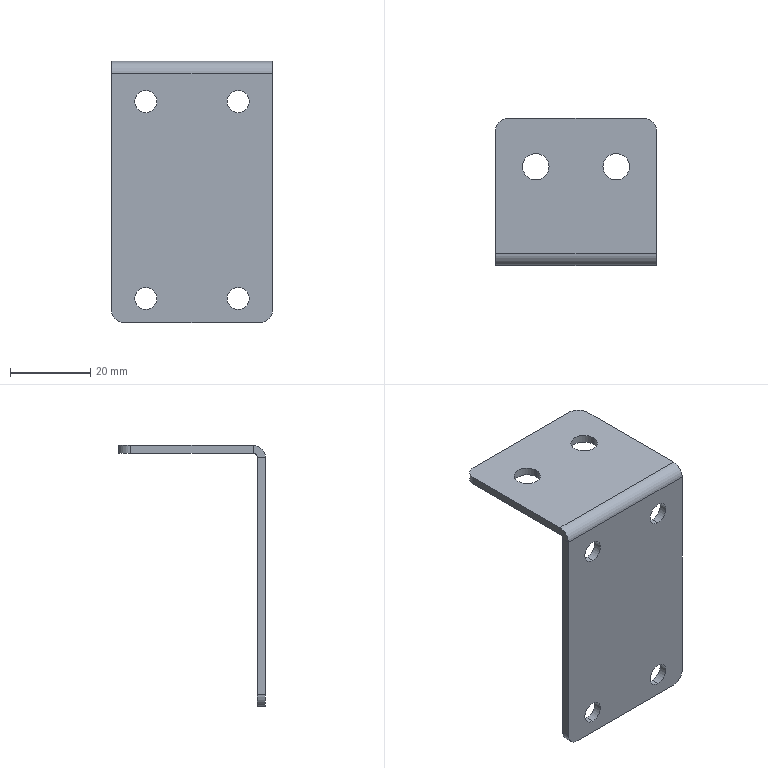Part | SolidWorks | features HoleWzd 2, Fillet 1, FlatPattern 1, SMBaseFlange 1, SheetMetal 1 | 1 solid | 30 faces | box 40 x 36.5 x 65 mm | volume 7549 mm3 | cylinder 18 | plane 12 | commonest cylinder face diameters 5.5 x8 6 x5 6.6 x4 2 x1
STEP:
#1=CARTESIAN_POINT('',(31.5,2.,-56.25));
#2=VERTEX_POINT('',#1);
#3=CARTESIAN_POINT('',(31.5,2.,-61.75));
#4=VERTEX_POINT('',#3);
#5=CARTESIAN_POINT('',(31.5,2.,-59.));
#6=DIRECTION('',(0.,-1.,0.));
#7=DIRECTION('',(0.,0.,-1.));
#8=AXIS2_PLACEMENT_3D('',#5,#6,#7);
#9=CIRCLE('',#8,2.75);
#10=EDGE_CURVE('',#2,#4,#9,.T.);
#11=ORIENTED_EDGE('',*,*,#10,.F.);
#12=CARTESIAN_POINT('',(31.5,0.,-56.25));
#13=VERTEX_POINT('',#12);
#14=CARTESIAN_POINT('',(31.5,0.,-56.25));
#15=DIRECTION('',(0.,-1.,0.));
#16=VECTOR('',#15,1000.);
#17=LINE('',#14,#16);
#18=EDGE_CURVE('',#2,#13,#17,.T.);
#19=ORIENTED_EDGE('',*,*,#18,.T.);
#20=CARTESIAN_POINT('',(31.5,0.,-61.75));
#21=VERTEX_POINT('',#20);
#22=CARTESIAN_POINT('',(31.5,0.,-59.));
#23=DIRECTION('',(0.,-1.,0.));
#24=DIRECTION('',(0.,0.,-1.));
#25=AXIS2_PLACEMENT_3D('',#22,#23,#24);
#26=CIRCLE('',#25,2.75);
#27=EDGE_CURVE('',#13,#21,#26,.T.);
#28=ORIENTED_EDGE('',*,*,#27,.T.);
#29=CARTESIAN_POINT('',(31.5,0.,-61.75));
#30=DIRECTION('',(0.,-1.,0.));
#31=VECTOR('',#30,1000.);
#32=LINE('',#29,#31);
#33=EDGE_CURVE('',#4,#21,#32,.T.);
#34=ORIENTED_EDGE('',*,*,#33,.F.);
#35=EDGE_LOOP('',(#11,#19,#28,#34));
#36=FACE_OUTER_BOUND('',#35,.T.);
#37=CARTESIAN_POINT('',(31.5,0.,-59.));
#38=DIRECTION('',(0.,-1.,0.));
#39=DIRECTION('',(0.,0.,-1.));
#40=AXIS2_PLACEMENT_3D('',#37,#38,#39);
#41=CYLINDRICAL_SURFACE('',#40,2.75);
#42=ADVANCED_FACE('',(#36),#41,.F.);
#43=CARTESIAN_POINT('',(31.5,2.,-7.25));
#44=VERTEX_POINT('',#43);
#45=CARTESIAN_POINT('',(31.5,2.,-12.75));
#46=VERTEX_POINT('',#45);
#47=CARTESIAN_POINT('',(31.5,2.,-10.));
#48=DIRECTION('',(0.,-1.,0.));
#49=DIRECTION('',(0.,0.,-1.));
#50=AXIS2_PLACEMENT_3D('',#47,#48,#49);
#51=CIRCLE('',#50,2.75);
#52=EDGE_CURVE('',#44,#46,#51,.T.);
#53=ORIENTED_EDGE('',*,*,#52,.F.);
#54=CARTESIAN_POINT('',(31.5,0.,-7.25));
#55=VERTEX_POINT('',#54);
#56=CARTESIAN_POINT('',(31.5,0.,-7.25));
#57=DIRECTION('',(0.,-1.,0.));
#58=VECTOR('',#57,1000.);
#59=LINE('',#56,#58);
#60=EDGE_CURVE('',#44,#55,#59,.T.);
#61=ORIENTED_EDGE('',*,*,#60,.T.);
#62=CARTESIAN_POINT('',(31.5,0.,-12.75));
#63=VERTEX_POINT('',#62);
#64=CARTESIAN_POINT('',(31.5,0.,-10.));
#65=DIRECTION('',(0.,-1.,0.));
#66=DIRECTION('',(0.,0.,-1.));
#67=AXIS2_PLACEMENT_3D('',#64,#65,#66);
#68=CIRCLE('',#67,2.75);
#69=EDGE_CURVE('',#55,#63,#68,.T.);
#70=ORIENTED_EDGE('',*,*,#69,.T.);
#71=CARTESIAN_POINT('',(31.5,0.,-12.75));
#72=DIRECTION('',(0.,-1.,0.));
#73=VECTOR('',#72,1000.);
#74=LINE('',#71,#73);
#75=EDGE_CURVE('',#46,#63,#74,.T.);
#76=ORIENTED_EDGE('',*,*,#75,.F.);
#77=EDGE_LOOP('',(#53,#61,#70,#76));
#78=FACE_OUTER_BOUND('',#77,.T.);
#79=CARTESIAN_POINT('',(31.5,0.,-10.));
#80=DIRECTION('',(0.,-1.,0.));
#81=DIRECTION('',(0.,0.,-1.));
#82=AXIS2_PLACEMENT_3D('',#79,#80,#81);
#83=CYLINDRICAL_SURFACE('',#82,2.75);
#84=ADVANCED_FACE('',(#78),#83,.F.);
#85=CARTESIAN_POINT('',(8.5,2.,-7.25));
#86=VERTEX_POINT('',#85);
#87=CARTESIAN_POINT('',(8.5,2.,-12.75));
#88=VERTEX_POINT('',#87);
#89=CARTESIAN_POINT('',(8.5,2.,-10.));
#90=DIRECTION('',(0.,-1.,0.));
#91=DIRECTION('',(0.,0.,-1.));
#92=AXIS2_PLACEMENT_3D('',#89,#90,#91);
#93=CIRCLE('',#92,2.75);
#94=EDGE_CURVE('',#86,#88,#93,.T.);
#95=ORIENTED_EDGE('',*,*,#94,.F.);
#96=CARTESIAN_POINT('',(8.5,0.,-7.25));
#97=VERTEX_POINT('',#96);
#98=CARTESIAN_POINT('',(8.5,0.,-7.25));
#99=DIRECTION('',(0.,-1.,0.));
#100=VECTOR('',#99,1000.);
#101=LINE('',#98,#100);
#102=EDGE_CURVE('',#86,#97,#101,.T.);
#103=ORIENTED_EDGE('',*,*,#102,.T.);
#104=CARTESIAN_POINT('',(8.5,0.,-12.75));
#105=VERTEX_POINT('',#104);
#106=CARTESIAN_POINT('',(8.5,0.,-10.));
#107=DIRECTION('',(0.,-1.,0.));
#108=DIRECTION('',(0.,0.,-1.));
#109=AXIS2_PLACEMENT_3D('',#106,#107,#108);
#110=CIRCLE('',#109,2.75);
#111=EDGE_CURVE('',#97,#105,#110,.T.);
#112=ORIENTED_EDGE('',*,*,#111,.T.);
#113=CARTESIAN_POINT('',(8.5,0.,-12.75));
#114=DIRECTION('',(0.,-1.,0.));
#115=VECTOR('',#114,1000.);
#116=LINE('',#113,#115);
#117=EDGE_CURVE('',#88,#105,#116,.T.);
#118=ORIENTED_EDGE('',*,*,#117,.F.);
#119=EDGE_LOOP('',(#95,#103,#112,#118));
#120=FACE_OUTER_BOUND('',#119,.T.);
#121=CARTESIAN_POINT('',(8.5,0.,-10.));
#122=DIRECTION('',(0.,-1.,0.));
#123=DIRECTION('',(0.,0.,-1.));
#124=AXIS2_PLACEMENT_3D('',#121,#122,#123);
#125=CYLINDRICAL_SURFACE('',#124,2.75);
#126=ADVANCED_FACE('',(#120),#125,.F.);
#127=CARTESIAN_POINT('',(8.5,2.,-56.25));
#128=VERTEX_POINT('',#127);
#129=CARTESIAN_POINT('',(8.5,2.,-61.75));
#130=VERTEX_POINT('',#129);
#131=CARTESIAN_POINT('',(8.5,2.,-59.));
#132=DIRECTION('',(0.,-1.,0.));
#133=DIRECTION('',(0.,0.,-1.));
#134=AXIS2_PLACEMENT_3D('',#131,#132,#133);
#135=CIRCLE('',#134,2.75);
#136=EDGE_CURVE('',#128,#130,#135,.T.);
#137=ORIENTED_EDGE('',*,*,#136,.F.);
#138=CARTESIAN_POINT('',(8.5,0.,-56.25));
#139=VERTEX_POINT('',#138);
#140=CARTESIAN_POINT('',(8.5,0.,-56.25));
#141=DIRECTION('',(0.,-1.,0.));
#142=VECTOR('',#141,1000.);
#143=LINE('',#140,#142);
#144=EDGE_CURVE('',#128,#139,#143,.T.);
#145=ORIENTED_EDGE('',*,*,#144,.T.);
#146=CARTESIAN_POINT('',(8.5,0.,-61.75));
#147=VERTEX_POINT('',#146);
#148=CARTESIAN_POINT('',(8.5,0.,-59.));
#149=DIRECTION('',(0.,-1.,0.));
#150=DIRECTION('',(0.,0.,-1.));
#151=AXIS2_PLACEMENT_3D('',#148,#149,#150);
#152=CIRCLE('',#151,2.75);
#153=EDGE_CURVE('',#139,#147,#152,.T.);
#154=ORIENTED_EDGE('',*,*,#153,.T.);
#155=CARTESIAN_POINT('',(8.5,0.,-61.75));
#156=DIRECTION('',(0.,-1.,0.));
#157=VECTOR('',#156,1000.);
#158=LINE('',#155,#157);
#159=EDGE_CURVE('',#130,#147,#158,.T.);
#160=ORIENTED_EDGE('',*,*,#159,.F.);
#161=EDGE_LOOP('',(#137,#145,#154,#160));
#162=FACE_OUTER_BOUND('',#161,.T.);
#163=CARTESIAN_POINT('',(8.5,0.,-59.));
#164=DIRECTION('',(0.,-1.,0.));
#165=DIRECTION('',(0.,0.,-1.));
#166=AXIS2_PLACEMENT_3D('',#163,#164,#165);
#167=CYLINDRICAL_SURFACE('',#166,2.75);
#168=ADVANCED_FACE('',(#162),#167,.F.);
#169=CARTESIAN_POINT('',(33.3,24.5,0.));
#170=VERTEX_POINT('',#169);
#171=CARTESIAN_POINT('',(26.7,24.5,0.));
#172=VERTEX_POINT('',#171);
#173=CARTESIAN_POINT('',(30.,24.5,0.));
#174=DIRECTION('',(0.,0.,-1.));
#175=DIRECTION('',(-1.,0.,0.));
#176=AXIS2_PLACEMENT_3D('',#173,#174,#175);
#177=CIRCLE('',#176,3.3);
#178=EDGE_CURVE('',#170,#172,#177,.T.);
#179=ORIENTED_EDGE('',*,*,#178,.F.);
#180=CARTESIAN_POINT('',(33.3,24.5,-2.));
#181=VERTEX_POINT('',#180);
#182=CARTESIAN_POINT('',(33.3,24.5,-2.));
#183=DIRECTION('',(0.,0.,-1.));
#184=VECTOR('',#183,1000.);
#185=LINE('',#182,#184);
#186=EDGE_CURVE('',#170,#181,#185,.T.);
#187=ORIENTED_EDGE('',*,*,#186,.T.);
#188=CARTESIAN_POINT('',(26.7,24.5,-2.));
#189=VERTEX_POINT('',#188);
#190=CARTESIAN_POINT('',(30.,24.5,-2.));
#191=DIRECTION('',(0.,0.,-1.));
#192=DIRECTION('',(-1.,0.,0.));
#193=AXIS2_PLACEMENT_3D('',#190,#191,#192);
#194=CIRCLE('',#193,3.3);
#195=EDGE_CURVE('',#181,#189,#194,.T.);
#196=ORIENTED_EDGE('',*,*,#195,.T.);
#197=CARTESIAN_POINT('',(26.7,24.5,-2.));
#198=DIRECTION('',(0.,0.,-1.));
#199=VECTOR('',#198,1000.);
#200=LINE('',#197,#199);
#201=EDGE_CURVE('',#172,#189,#200,.T.);
#202=ORIENTED_EDGE('',*,*,#201,.F.);
#203=EDGE_LOOP('',(#179,#187,#196,#202));
#204=FACE_OUTER_BOUND('',#203,.T.);
#205=CARTESIAN_POINT('',(30.,24.5,-2.));
#206=DIRECTION('',(0.,0.,-1.));
#207=DIRECTION('',(-1.,0.,0.));
#208=AXIS2_PLACEMENT_3D('',#205,#206,#207);
#209=CYLINDRICAL_SURFACE('',#208,3.3);
#210=ADVANCED_FACE('',(#204),#209,.F.);
#211=CARTESIAN_POINT('',(13.3,24.5,0.));
#212=VERTEX_POINT('',#211);
#213=CARTESIAN_POINT('',(6.7,24.5,0.));
#214=VERTEX_POINT('',#213);
#215=CARTESIAN_POINT('',(10.,24.5,0.));
#216=DIRECTION('',(0.,0.,-1.));
#217=DIRECTION('',(-1.,0.,0.));
#218=AXIS2_PLACEMENT_3D('',#215,#216,#217);
#219=CIRCLE('',#218,3.3);
#220=EDGE_CURVE('',#212,#214,#219,.T.);
#221=ORIENTED_EDGE('',*,*,#220,.F.);
#222=CARTESIAN_POINT('',(13.3,24.5,-2.));
#223=VERTEX_POINT('',#222);
#224=CARTESIAN_POINT('',(13.3,24.5,-2.));
#225=DIRECTION('',(0.,0.,-1.));
#226=VECTOR('',#225,1000.);
#227=LINE('',#224,#226);
#228=EDGE_CURVE('',#212,#223,#227,.T.);
#229=ORIENTED_EDGE('',*,*,#228,.T.);
#230=CARTESIAN_POINT('',(6.7,24.5,-2.));
#231=VERTEX_POINT('',#230);
#232=CARTESIAN_POINT('',(10.,24.5,-2.));
#233=DIRECTION('',(0.,0.,-1.));
#234=DIRECTION('',(-1.,0.,0.));
#235=AXIS2_PLACEMENT_3D('',#232,#233,#234);
#236=CIRCLE('',#235,3.3);
#237=EDGE_CURVE('',#223,#231,#236,.T.);
#238=ORIENTED_EDGE('',*,*,#237,.T.);
#239=CARTESIAN_POINT('',(6.7,24.5,-2.));
#240=DIRECTION('',(0.,0.,-1.));
#241=VECTOR('',#240,1000.);
#242=LINE('',#239,#241);
#243=EDGE_CURVE('',#214,#231,#242,.T.);
#244=ORIENTED_EDGE('',*,*,#243,.F.);
#245=EDGE_LOOP('',(#221,#229,#238,#244));
#246=FACE_OUTER_BOUND('',#245,.T.);
#247=CARTESIAN_POINT('',(10.,24.5,-2.));
#248=DIRECTION('',(0.,0.,-1.));
#249=DIRECTION('',(-1.,0.,0.));
#250=AXIS2_PLACEMENT_3D('',#247,#248,#249);
#251=CYLINDRICAL_SURFACE('',#250,3.3);
#252=ADVANCED_FACE('',(#246),#251,.F.);
#253=CARTESIAN_POINT('',(40.,3.,0.));
#254=VERTEX_POINT('',#253);
#255=CARTESIAN_POINT('',(40.,3.,-2.));
#256=VERTEX_POINT('',#255);
#257=CARTESIAN_POINT('',(40.,3.,0.));
#258=DIRECTION('',(0.,0.,-1.));
#259=VECTOR('',#258,1000.);
#260=LINE('',#257,#259);
#261=EDGE_CURVE('',#254,#256,#260,.T.);
#262=ORIENTED_EDGE('',*,*,#261,.F.);
#263=CARTESIAN_POINT('',(40.,0.,-3.));
#264=VERTEX_POINT('',#263);
#265=CARTESIAN_POINT('',(40.,3.,-3.));
#266=DIRECTION('',(-1.,0.,0.));
#267=DIRECTION('',(0.,0.,-1.));
#268=AXIS2_PLACEMENT_3D('',#265,#266,#267);
#269=CIRCLE('',#268,3.);
#270=EDGE_CURVE('',#264,#254,#269,.T.);
#271=ORIENTED_EDGE('',*,*,#270,.F.);
#272=CARTESIAN_POINT('',(40.,2.,-3.));
#273=VERTEX_POINT('',#272);
#274=CARTESIAN_POINT('',(40.,2.,-3.));
#275=DIRECTION('',(0.,-1.,0.));
#276=VECTOR('',#275,1000.);
#277=LINE('',#274,#276);
#278=EDGE_CURVE('',#273,#264,#277,.T.);
#279=ORIENTED_EDGE('',*,*,#278,.F.);
#280=CARTESIAN_POINT('',(40.,3.,-3.));
#281=DIRECTION('',(-1.,0.,0.));
#282=DIRECTION('',(0.,0.,-1.));
#283=AXIS2_PLACEMENT_3D('',#280,#281,#282);
#284=CIRCLE('',#283,1.);
#285=EDGE_CURVE('',#273,#256,#284,.T.);
#286=ORIENTED_EDGE('',*,*,#285,.T.);
#287=EDGE_LOOP('',(#262,#271,#279,#286));
#288=FACE_OUTER_BOUND('',#287,.T.);
#289=CARTESIAN_POINT('',(40.,3.,0.));
#290=DIRECTION('',(1.,0.,0.));
#291=DIRECTION('',(0.,0.,-1.));
#292=AXIS2_PLACEMENT_3D('',#289,#290,#291);
#293=PLANE('',#292);
#294=ADVANCED_FACE('',(#288),#293,.T.);
#295=CARTESIAN_POINT('',(40.,33.5,-2.));
#296=VERTEX_POINT('',#295);
#297=CARTESIAN_POINT('',(40.,0.,-2.));
#298=DIRECTION('',(0.,1.,0.));
#299=VECTOR('',#298,1000.);
#300=LINE('',#297,#299);
#301=EDGE_CURVE('',#256,#296,#300,.T.);
#302=ORIENTED_EDGE('',*,*,#301,.T.);
#303=CARTESIAN_POINT('',(40.,33.5,0.));
#304=VERTEX_POINT('',#303);
#305=CARTESIAN_POINT('',(40.,33.5,-3.));
#306=DIRECTION('',(0.,0.,1.));
#307=VECTOR('',#306,1000.);
#308=LINE('',#305,#307);
#309=EDGE_CURVE('',#296,#304,#308,.T.);
#310=ORIENTED_EDGE('',*,*,#309,.T.);
#311=CARTESIAN_POINT('',(40.,0.,0.));
#312=DIRECTION('',(0.,1.,0.));
#313=VECTOR('',#312,1000.);
#314=LINE('',#311,#313);
#315=EDGE_CURVE('',#254,#304,#314,.T.);
#316=ORIENTED_EDGE('',*,*,#315,.F.);
#317=ORIENTED_EDGE('',*,*,#261,.T.);
#318=EDGE_LOOP('',(#302,#310,#316,#317));
#319=FACE_OUTER_BOUND('',#318,.T.);
#320=CARTESIAN_POINT('',(40.,2.,-3.));
#321=DIRECTION('',(1.,0.,0.));
#322=DIRECTION('',(0.,0.,-1.));
#323=AXIS2_PLACEMENT_3D('',#320,#321,#322);
#324=PLANE('',#323);
#325=ADVANCED_FACE('',(#319),#324,.T.);
#326=CARTESIAN_POINT('',(0.,0.,-3.));
#327=VERTEX_POINT('',#326);
#328=CARTESIAN_POINT('',(0.,2.,-3.));
#329=VERTEX_POINT('',#328);
#330=CARTESIAN_POINT('',(0.,0.,-3.));
#331=DIRECTION('',(0.,1.,0.));
#332=VECTOR('',#331,1000.);
#333=LINE('',#330,#332);
#334=EDGE_CURVE('',#327,#329,#333,.T.);
#335=ORIENTED_EDGE('',*,*,#334,.F.);
#336=CARTESIAN_POINT('',(0.,3.,0.));
#337=VERTEX_POINT('',#336);
#338=CARTESIAN_POINT('',(0.,3.,-3.));
#339=DIRECTION('',(-1.,0.,0.));
#340=DIRECTION('',(0.,0.,-1.));
#341=AXIS2_PLACEMENT_3D('',#338,#339,#340);
#342=CIRCLE('',#341,3.);
#343=EDGE_CURVE('',#327,#337,#342,.T.);
#344=ORIENTED_EDGE('',*,*,#343,.T.);
#345=CARTESIAN_POINT('',(0.,3.,-2.));
#346=VERTEX_POINT('',#345);
#347=CARTESIAN_POINT('',(0.,3.,-2.));
#348=DIRECTION('',(0.,0.,1.));
#349=VECTOR('',#348,1000.);
#350=LINE('',#347,#349);
#351=EDGE_CURVE('',#346,#337,#350,.T.);
#352=ORIENTED_EDGE('',*,*,#351,.F.);
#353=CARTESIAN_POINT('',(0.,3.,-3.));
#354=DIRECTION('',(-1.,0.,0.));
#355=DIRECTION('',(0.,0.,-1.));
#356=AXIS2_PLACEMENT_3D('',#353,#354,#355);
#357=CIRCLE('',#356,1.);
#358=EDGE_CURVE('',#329,#346,#357,.T.);
#359=ORIENTED_EDGE('',*,*,#358,.F.);
#360=EDGE_LOOP('',(#335,#344,#352,#359));
#361=FACE_OUTER_BOUND('',#360,.T.);
#362=CARTESIAN_POINT('',(0.,0.,-3.));
#363=DIRECTION('',(-1.,0.,0.));
#364=DIRECTION('',(0.,0.,1.));
#365=AXIS2_PLACEMENT_3D('',#362,#363,#364);
#366=PLANE('',#365);
#367=ADVANCED_FACE('',(#361),#366,.T.);
#368=CARTESIAN_POINT('',(0.,2.,-62.));
#369=VERTEX_POINT('',#368);
#370=CARTESIAN_POINT('',(0.,2.,0.));
#371=DIRECTION('',(0.,0.,1.));
#372=VECTOR('',#371,1000.);
#373=LINE('',#370,#372);
#374=EDGE_CURVE('',#369,#329,#373,.T.);
#375=ORIENTED_EDGE('',*,*,#374,.F.);
#376=CARTESIAN_POINT('',(0.,0.,-62.));
#377=VERTEX_POINT('',#376);
#378=CARTESIAN_POINT('',(0.,3.,-62.));
#379=DIRECTION('',(0.,-1.,0.));
#380=VECTOR('',#379,1000.);
#381=LINE('',#378,#380);
#382=EDGE_CURVE('',#369,#377,#381,.T.);
#383=ORIENTED_EDGE('',*,*,#382,.T.);
#384=CARTESIAN_POINT('',(0.,0.,0.));
#385=DIRECTION('',(0.,0.,1.));
#386=VECTOR('',#385,1000.);
#387=LINE('',#384,#386);
#388=EDGE_CURVE('',#377,#327,#387,.T.);
#389=ORIENTED_EDGE('',*,*,#388,.T.);
#390=ORIENTED_EDGE('',*,*,#334,.T.);
#391=EDGE_LOOP('',(#375,#383,#389,#390));
#392=FACE_OUTER_BOUND('',#391,.T.);
#393=CARTESIAN_POINT('',(0.,3.,-2.));
#394=DIRECTION('',(-1.,0.,0.));
#395=DIRECTION('',(0.,0.,1.));
#396=AXIS2_PLACEMENT_3D('',#393,#394,#395);
#397=PLANE('',#396);
#398=ADVANCED_FACE('',(#392),#397,.T.);
#399=CARTESIAN_POINT('',(30.,24.5,-2.));
#400=DIRECTION('',(0.,0.,-1.));
#401=DIRECTION('',(-1.,0.,0.));
#402=AXIS2_PLACEMENT_3D('',#399,#400,#401);
#403=CIRCLE('',#402,3.3);
#404=EDGE_CURVE('',#189,#181,#403,.T.);
#405=ORIENTED_EDGE('',*,*,#404,.F.);
#406=ORIENTED_EDGE('',*,*,#195,.F.);
#407=EDGE_LOOP('',(#405,#406));
#408=FACE_BOUND('',#407,.T.);
#409=CARTESIAN_POINT('',(10.,24.5,-2.));
#410=DIRECTION('',(0.,0.,-1.));
#411=DIRECTION('',(-1.,0.,0.));
#412=AXIS2_PLACEMENT_3D('',#409,#410,#411);
#413=CIRCLE('',#412,3.3);
#414=EDGE_CURVE('',#231,#223,#413,.T.);
#415=ORIENTED_EDGE('',*,*,#414,.F.);
#416=ORIENTED_EDGE('',*,*,#237,.F.);
#417=EDGE_LOOP('',(#415,#416));
#418=FACE_BOUND('',#417,.T.);
#419=CARTESIAN_POINT('',(37.,36.5,-2.));
#420=VERTEX_POINT('',#419);
#421=CARTESIAN_POINT('',(3.,36.5,-2.));
#422=VERTEX_POINT('',#421);
#423=CARTESIAN_POINT('',(40.,36.5,-2.));
#424=DIRECTION('',(-1.,0.,0.));
#425=VECTOR('',#424,1000.);
#426=LINE('',#423,#425);
#427=EDGE_CURVE('',#420,#422,#426,.T.);
#428=ORIENTED_EDGE('',*,*,#427,.F.);
#429=CARTESIAN_POINT('',(37.,33.5,-2.));
#430=DIRECTION('',(0.,0.,-1.));
#431=DIRECTION('',(1.,0.,0.));
#432=AXIS2_PLACEMENT_3D('',#429,#430,#431);
#433=CIRCLE('',#432,3.);
#434=EDGE_CURVE('',#420,#296,#433,.T.);
#435=ORIENTED_EDGE('',*,*,#434,.T.);
#436=ORIENTED_EDGE('',*,*,#301,.F.);
#437=CARTESIAN_POINT('',(40.,3.,-2.));
#438=DIRECTION('',(-1.,0.,0.));
#439=VECTOR('',#438,1000.);
#440=LINE('',#437,#439);
#441=EDGE_CURVE('',#256,#346,#440,.T.);
#442=ORIENTED_EDGE('',*,*,#441,.T.);
#443=CARTESIAN_POINT('',(0.,33.5,-2.));
#444=VERTEX_POINT('',#443);
#445=CARTESIAN_POINT('',(0.,0.,-2.));
#446=DIRECTION('',(0.,1.,0.));
#447=VECTOR('',#446,1000.);
#448=LINE('',#445,#447);
#449=EDGE_CURVE('',#346,#444,#448,.T.);
#450=ORIENTED_EDGE('',*,*,#449,.T.);
#451=CARTESIAN_POINT('',(3.,33.5,-2.));
#452=DIRECTION('',(0.,0.,-1.));
#453=DIRECTION('',(1.,0.,0.));
#454=AXIS2_PLACEMENT_3D('',#451,#452,#453);
#455=CIRCLE('',#454,3.);
#456=EDGE_CURVE('',#444,#422,#455,.T.);
#457=ORIENTED_EDGE('',*,*,#456,.T.);
#458=EDGE_LOOP('',(#428,#435,#436,#442,#450,#457));
#459=FACE_OUTER_BOUND('',#458,.T.);
#460=CARTESIAN_POINT('',(40.,0.,-2.));
#461=DIRECTION('',(0.,0.,1.));
#462=DIRECTION('',(1.,0.,0.));
#463=AXIS2_PLACEMENT_3D('',#460,#461,#462);
#464=PLANE('',#463);
#465=ADVANCED_FACE('',(#408,#418,#459),#464,.F.);
#466=CARTESIAN_POINT('',(37.,36.5,0.));
#467=VERTEX_POINT('',#466);
#468=CARTESIAN_POINT('',(3.,36.5,0.));
#469=VERTEX_POINT('',#468);
#470=CARTESIAN_POINT('',(40.,36.5,0.));
#471=DIRECTION('',(-1.,0.,0.));
#472=VECTOR('',#471,1000.);
#473=LINE('',#470,#472);
#474=EDGE_CURVE('',#467,#469,#473,.T.);
#475=ORIENTED_EDGE('',*,*,#474,.F.);
#476=CARTESIAN_POINT('',(37.,36.5,0.));
#477=DIRECTION('',(0.,0.,-1.));
#478=VECTOR('',#477,1000.);
#479=LINE('',#476,#478);
#480=EDGE_CURVE('',#467,#420,#479,.T.);
#481=ORIENTED_EDGE('',*,*,#480,.T.);
#482=ORIENTED_EDGE('',*,*,#427,.T.);
#483=CARTESIAN_POINT('',(3.,36.5,0.));
#484=DIRECTION('',(0.,0.,1.));
#485=VECTOR('',#484,1000.);
#486=LINE('',#483,#485);
#487=EDGE_CURVE('',#422,#469,#486,.T.);
#488=ORIENTED_EDGE('',*,*,#487,.T.);
#489=EDGE_LOOP('',(#475,#481,#482,#488));
#490=FACE_OUTER_BOUND('',#489,.T.);
#491=CARTESIAN_POINT('',(40.,36.5,0.));
#492=DIRECTION('',(0.,1.,0.));
#493=DIRECTION('',(0.,0.,1.));
#494=AXIS2_PLACEMENT_3D('',#491,#492,#493);
#495=PLANE('',#494);
#496=ADVANCED_FACE('',(#490),#495,.T.);
#497=CARTESIAN_POINT('',(30.,24.5,0.));
#498=DIRECTION('',(0.,0.,-1.));
#499=DIRECTION('',(-1.,0.,0.));
#500=AXIS2_PLACEMENT_3D('',#497,#498,#499);
#501=CIRCLE('',#500,3.3);
#502=EDGE_CURVE('',#172,#170,#501,.T.);
#503=ORIENTED_EDGE('',*,*,#502,.T.);
#504=ORIENTED_EDGE('',*,*,#178,.T.);
#505=EDGE_LOOP('',(#503,#504));
#506=FACE_BOUND('',#505,.T.);
#507=CARTESIAN_POINT('',(10.,24.5,0.));
#508=DIRECTION('',(0.,0.,-1.));
#509=DIRECTION('',(-1.,0.,0.));
#510=AXIS2_PLACEMENT_3D('',#507,#508,#509);
#511=CIRCLE('',#510,3.3);
#512=EDGE_CURVE('',#214,#212,#511,.T.);
#513=ORIENTED_EDGE('',*,*,#512,.T.);
#514=ORIENTED_EDGE('',*,*,#220,.T.);
#515=EDGE_LOOP('',(#513,#514));
#516=FACE_BOUND('',#515,.T.);
#517=ORIENTED_EDGE('',*,*,#315,.T.);
#518=CARTESIAN_POINT('',(37.,33.5,0.));
#519=DIRECTION('',(0.,0.,1.));
#520=DIRECTION('',(1.,0.,0.));
#521=AXIS2_PLACEMENT_3D('',#518,#519,#520);
#522=CIRCLE('',#521,3.);
#523=EDGE_CURVE('',#304,#467,#522,.T.);
#524=ORIENTED_EDGE('',*,*,#523,.T.);
#525=ORIENTED_EDGE('',*,*,#474,.T.);
#526=CARTESIAN_POINT('',(0.,33.5,0.));
#527=VERTEX_POINT('',#526);
#528=CARTESIAN_POINT('',(3.,33.5,0.));
#529=DIRECTION('',(0.,0.,1.));
#530=DIRECTION('',(1.,0.,0.));
#531=AXIS2_PLACEMENT_3D('',#528,#529,#530);
#532=CIRCLE('',#531,3.);
#533=EDGE_CURVE('',#469,#527,#532,.T.);
#534=ORIENTED_EDGE('',*,*,#533,.T.);
#535=CARTESIAN_POINT('',(0.,0.,0.));
#536=DIRECTION('',(0.,1.,0.));
#537=VECTOR('',#536,1000.);
#538=LINE('',#535,#537);
#539=EDGE_CURVE('',#337,#527,#538,.T.);
#540=ORIENTED_EDGE('',*,*,#539,.F.);
#541=CARTESIAN_POINT('',(40.,3.,0.));
#542=DIRECTION('',(-1.,0.,0.));
#543=VECTOR('',#542,1000.);
#544=LINE('',#541,#543);
#545=EDGE_CURVE('',#254,#337,#544,.T.);
#546=ORIENTED_EDGE('',*,*,#545,.F.);
#547=EDGE_LOOP('',(#517,#524,#525,#534,#540,#546));
#548=FACE_OUTER_BOUND('',#547,.T.);
#549=CARTESIAN_POINT('',(40.,0.,0.));
#550=DIRECTION('',(0.,0.,1.));
#551=DIRECTION('',(1.,0.,0.));
#552=AXIS2_PLACEMENT_3D('',#549,#550,#551);
#553=PLANE('',#552);
#554=ADVANCED_FACE('',(#506,#516,#548),#553,.T.);
#555=ORIENTED_EDGE('',*,*,#343,.F.);
#556=CARTESIAN_POINT('',(40.,0.,-3.));
#557=DIRECTION('',(-1.,0.,0.));
#558=VECTOR('',#557,1000.);
#559=LINE('',#556,#558);
#560=EDGE_CURVE('',#264,#327,#559,.T.);
#561=ORIENTED_EDGE('',*,*,#560,.F.);
#562=ORIENTED_EDGE('',*,*,#270,.T.);
#563=ORIENTED_EDGE('',*,*,#545,.T.);
#564=EDGE_LOOP('',(#555,#561,#562,#563));
#565=FACE_OUTER_BOUND('',#564,.T.);
#566=CARTESIAN_POINT('',(40.,3.,-3.));
#567=DIRECTION('',(-1.,0.,0.));
#568=DIRECTION('',(0.,0.,1.));
#569=AXIS2_PLACEMENT_3D('',#566,#567,#568);
#570=CYLINDRICAL_SURFACE('',#569,3.);
#571=ADVANCED_FACE('',(#565),#570,.T.);
#572=CARTESIAN_POINT('',(31.5,0.,-59.));
#573=DIRECTION('',(0.,-1.,0.));
#574=DIRECTION('',(0.,0.,-1.));
#575=AXIS2_PLACEMENT_3D('',#572,#573,#574);
#576=CIRCLE('',#575,2.75);
#577=EDGE_CURVE('',#21,#13,#576,.T.);
#578=ORIENTED_EDGE('',*,*,#577,.F.);
#579=ORIENTED_EDGE('',*,*,#27,.F.);
#580=EDGE_LOOP('',(#578,#579));
#581=FACE_BOUND('',#580,.T.);
#582=CARTESIAN_POINT('',(31.5,0.,-10.));
#583=DIRECTION('',(0.,-1.,0.));
#584=DIRECTION('',(0.,0.,-1.));
#585=AXIS2_PLACEMENT_3D('',#582,#583,#584);
#586=CIRCLE('',#585,2.75);
#587=EDGE_CURVE('',#63,#55,#586,.T.);
#588=ORIENTED_EDGE('',*,*,#587,.F.);
#589=ORIENTED_EDGE('',*,*,#69,.F.);
#590=EDGE_LOOP('',(#588,#589));
#591=FACE_BOUND('',#590,.T.);
#592=CARTESIAN_POINT('',(8.5,0.,-10.));
#593=DIRECTION('',(0.,-1.,0.));
#594=DIRECTION('',(0.,0.,-1.));
#595=AXIS2_PLACEMENT_3D('',#592,#593,#594);
#596=CIRCLE('',#595,2.75);
#597=EDGE_CURVE('',#105,#97,#596,.T.);
#598=ORIENTED_EDGE('',*,*,#597,.F.);
#599=ORIENTED_EDGE('',*,*,#111,.F.);
#600=EDGE_LOOP('',(#598,#599));
#601=FACE_BOUND('',#600,.T.);
#602=CARTESIAN_POINT('',(8.5,0.,-59.));
#603=DIRECTION('',(0.,-1.,0.));
#604=DIRECTION('',(0.,0.,-1.));
#605=AXIS2_PLACEMENT_3D('',#602,#603,#604);
#606=CIRCLE('',#605,2.75);
#607=EDGE_CURVE('',#147,#139,#606,.T.);
#608=ORIENTED_EDGE('',*,*,#607,.F.);
#609=ORIENTED_EDGE('',*,*,#153,.F.);
#610=EDGE_LOOP('',(#608,#609));
#611=FACE_BOUND('',#610,.T.);
#612=ORIENTED_EDGE('',*,*,#388,.F.);
#613=CARTESIAN_POINT('',(3.,0.,-65.));
#614=VERTEX_POINT('',#613);
#615=CARTESIAN_POINT('',(3.,0.,-62.));
#616=DIRECTION('',(0.,-1.,0.));
#617=DIRECTION('',(0.,0.,-1.));
#618=AXIS2_PLACEMENT_3D('',#615,#616,#617);
#619=CIRCLE('',#618,3.);
#620=EDGE_CURVE('',#377,#614,#619,.T.);
#621=ORIENTED_EDGE('',*,*,#620,.T.);
#622=CARTESIAN_POINT('',(37.,0.,-65.));
#623=VERTEX_POINT('',#622);
#624=CARTESIAN_POINT('',(40.,0.,-65.));
#625=DIRECTION('',(-1.,0.,0.));
#626=VECTOR('',#625,1000.);
#627=LINE('',#624,#626);
#628=EDGE_CURVE('',#623,#614,#627,.T.);
#629=ORIENTED_EDGE('',*,*,#628,.F.);
#630=CARTESIAN_POINT('',(40.,0.,-62.));
#631=VERTEX_POINT('',#630);
#632=CARTESIAN_POINT('',(37.,0.,-62.));
#633=DIRECTION('',(0.,-1.,0.));
#634=DIRECTION('',(0.,0.,-1.));
#635=AXIS2_PLACEMENT_3D('',#632,#633,#634);
#636=CIRCLE('',#635,3.);
#637=EDGE_CURVE('',#623,#631,#636,.T.);
#638=ORIENTED_EDGE('',*,*,#637,.T.);
#639=CARTESIAN_POINT('',(40.,0.,0.));
#640=DIRECTION('',(0.,0.,1.));
#641=VECTOR('',#640,1000.);
#642=LINE('',#639,#641);
#643=EDGE_CURVE('',#631,#264,#642,.T.);
#644=ORIENTED_EDGE('',*,*,#643,.T.);
#645=ORIENTED_EDGE('',*,*,#560,.T.);
#646=EDGE_LOOP('',(#612,#621,#629,#638,#644,#645));
#647=FACE_OUTER_BOUND('',#646,.T.);
#648=CARTESIAN_POINT('',(40.,0.,0.));
#649=DIRECTION('',(0.,-1.,0.));
#650=DIRECTION('',(0.,0.,-1.));
#651=AXIS2_PLACEMENT_3D('',#648,#649,#650);
#652=PLANE('',#651);
#653=ADVANCED_FACE('',(#581,#591,#601,#611,#647),#652,.T.);
#654=ORIENTED_EDGE('',*,*,#628,.T.);
#655=CARTESIAN_POINT('',(3.,2.,-65.));
#656=VERTEX_POINT('',#655);
#657=CARTESIAN_POINT('',(3.,2.,-65.));
#658=DIRECTION('',(0.,1.,0.));
#659=VECTOR('',#658,1000.);
#660=LINE('',#657,#659);
#661=EDGE_CURVE('',#614,#656,#660,.T.);
#662=ORIENTED_EDGE('',*,*,#661,.T.);
#663=CARTESIAN_POINT('',(37.,2.,-65.));
#664=VERTEX_POINT('',#663);
#665=CARTESIAN_POINT('',(40.,2.,-65.));
#666=DIRECTION('',(-1.,0.,0.));
#667=VECTOR('',#666,1000.);
#668=LINE('',#665,#667);
#669=EDGE_CURVE('',#664,#656,#668,.T.);
#670=ORIENTED_EDGE('',*,*,#669,.F.);
#671=CARTESIAN_POINT('',(37.,2.,-65.));
#672=DIRECTION('',(0.,-1.,0.));
#673=VECTOR('',#672,1000.);
#674=LINE('',#671,#673);
#675=EDGE_CURVE('',#664,#623,#674,.T.);
#676=ORIENTED_EDGE('',*,*,#675,.T.);
#677=EDGE_LOOP('',(#654,#662,#670,#676));
#678=FACE_OUTER_BOUND('',#677,.T.);
#679=CARTESIAN_POINT('',(40.,2.,-65.));
#680=DIRECTION('',(0.,0.,-1.));
#681=DIRECTION('',(-1.,0.,0.));
#682=AXIS2_PLACEMENT_3D('',#679,#680,#681);
#683=PLANE('',#682);
#684=ADVANCED_FACE('',(#678),#683,.T.);
#685=CARTESIAN_POINT('',(31.5,2.,-59.));
#686=DIRECTION('',(0.,-1.,0.));
#687=DIRECTION('',(0.,0.,-1.));
#688=AXIS2_PLACEMENT_3D('',#685,#686,#687);
#689=CIRCLE('',#688,2.75);
#690=EDGE_CURVE('',#4,#2,#689,.T.);
#691=ORIENTED_EDGE('',*,*,#690,.T.);
#692=ORIENTED_EDGE('',*,*,#10,.T.);
#693=EDGE_LOOP('',(#691,#692));
#694=FACE_BOUND('',#693,.T.);
#695=CARTESIAN_POINT('',(31.5,2.,-10.));
#696=DIRECTION('',(0.,-1.,0.));
#697=DIRECTION('',(0.,0.,-1.));
#698=AXIS2_PLACEMENT_3D('',#695,#696,#697);
#699=CIRCLE('',#698,2.75);
#700=EDGE_CURVE('',#46,#44,#699,.T.);
#701=ORIENTED_EDGE('',*,*,#700,.T.);
#702=ORIENTED_EDGE('',*,*,#52,.T.);
#703=EDGE_LOOP('',(#701,#702));
#704=FACE_BOUND('',#703,.T.);
#705=CARTESIAN_POINT('',(8.5,2.,-10.));
#706=DIRECTION('',(0.,-1.,0.));
#707=DIRECTION('',(0.,0.,-1.));
#708=AXIS2_PLACEMENT_3D('',#705,#706,#707);
#709=CIRCLE('',#708,2.75);
#710=EDGE_CURVE('',#88,#86,#709,.T.);
#711=ORIENTED_EDGE('',*,*,#710,.T.);
#712=ORIENTED_EDGE('',*,*,#94,.T.);
#713=EDGE_LOOP('',(#711,#712));
#714=FACE_BOUND('',#713,.T.);
#715=CARTESIAN_POINT('',(8.5,2.,-59.));
#716=DIRECTION('',(0.,-1.,0.));
#717=DIRECTION('',(0.,0.,-1.));
#718=AXIS2_PLACEMENT_3D('',#715,#716,#717);
#719=CIRCLE('',#718,2.75);
#720=EDGE_CURVE('',#130,#128,#719,.T.);
#721=ORIENTED_EDGE('',*,*,#720,.T.);
#722=ORIENTED_EDGE('',*,*,#136,.T.);
#723=EDGE_LOOP('',(#721,#722));
#724=FACE_BOUND('',#723,.T.);
#725=ORIENTED_EDGE('',*,*,#669,.T.);
#726=CARTESIAN_POINT('',(3.,2.,-62.));
#727=DIRECTION('',(0.,1.,0.));
#728=DIRECTION('',(0.,0.,-1.));
#729=AXIS2_PLACEMENT_3D('',#726,#727,#728);
#730=CIRCLE('',#729,3.);
#731=EDGE_CURVE('',#656,#369,#730,.T.);
#732=ORIENTED_EDGE('',*,*,#731,.T.);
#733=ORIENTED_EDGE('',*,*,#374,.T.);
#734=CARTESIAN_POINT('',(40.,2.,-3.));
#735=DIRECTION('',(-1.,0.,0.));
#736=VECTOR('',#735,1000.);
#737=LINE('',#734,#736);
#738=EDGE_CURVE('',#273,#329,#737,.T.);
#739=ORIENTED_EDGE('',*,*,#738,.F.);
#740=CARTESIAN_POINT('',(40.,2.,-62.));
#741=VERTEX_POINT('',#740);
#742=CARTESIAN_POINT('',(40.,2.,0.));
#743=DIRECTION('',(0.,0.,1.));
#744=VECTOR('',#743,1000.);
#745=LINE('',#742,#744);
#746=EDGE_CURVE('',#741,#273,#745,.T.);
#747=ORIENTED_EDGE('',*,*,#746,.F.);
#748=CARTESIAN_POINT('',(37.,2.,-62.));
#749=DIRECTION('',(0.,1.,0.));
#750=DIRECTION('',(0.,0.,-1.));
#751=AXIS2_PLACEMENT_3D('',#748,#749,#750);
#752=CIRCLE('',#751,3.);
#753=EDGE_CURVE('',#741,#664,#752,.T.);
#754=ORIENTED_EDGE('',*,*,#753,.T.);
#755=EDGE_LOOP('',(#725,#732,#733,#739,#747,#754));
#756=FACE_OUTER_BOUND('',#755,.T.);
#757=CARTESIAN_POINT('',(40.,2.,0.));
#758=DIRECTION('',(0.,-1.,0.));
#759=DIRECTION('',(0.,0.,-1.));
#760=AXIS2_PLACEMENT_3D('',#757,#758,#759);
#761=PLANE('',#760);
#762=ADVANCED_FACE('',(#694,#704,#714,#724,#756),#761,.F.);
#763=ORIENTED_EDGE('',*,*,#358,.T.);
#764=ORIENTED_EDGE('',*,*,#441,.F.);
#765=ORIENTED_EDGE('',*,*,#285,.F.);
#766=ORIENTED_EDGE('',*,*,#738,.T.);
#767=EDGE_LOOP('',(#763,#764,#765,#766));
#768=FACE_OUTER_BOUND('',#767,.T.);
#769=CARTESIAN_POINT('',(40.,3.,-3.));
#770=DIRECTION('',(-1.,0.,0.));
#771=DIRECTION('',(0.,0.,1.));
#772=AXIS2_PLACEMENT_3D('',#769,#770,#771);
#773=CYLINDRICAL_SURFACE('',#772,1.);
#774=ADVANCED_FACE('',(#768),#773,.F.);
#775=ORIENTED_EDGE('',*,*,#643,.F.);
#776=CARTESIAN_POINT('',(40.,3.,-62.));
#777=DIRECTION('',(0.,1.,0.));
#778=VECTOR('',#777,1000.);
#779=LINE('',#776,#778);
#780=EDGE_CURVE('',#631,#741,#779,.T.);
#781=ORIENTED_EDGE('',*,*,#780,.T.);
#782=ORIENTED_EDGE('',*,*,#746,.T.);
#783=ORIENTED_EDGE('',*,*,#278,.T.);
#784=EDGE_LOOP('',(#775,#781,#782,#783));
#785=FACE_OUTER_BOUND('',#784,.T.);
#786=CARTESIAN_POINT('',(40.,3.,-3.));
#787=DIRECTION('',(1.,0.,0.));
#788=DIRECTION('',(0.,0.,-1.));
#789=AXIS2_PLACEMENT_3D('',#786,#787,#788);
#790=PLANE('',#789);
#791=ADVANCED_FACE('',(#785),#790,.T.);
#792=ORIENTED_EDGE('',*,*,#539,.T.);
#793=CARTESIAN_POINT('',(0.,33.5,-2.));
#794=DIRECTION('',(0.,0.,-1.));
#795=VECTOR('',#794,1000.);
#796=LINE('',#793,#795);
#797=EDGE_CURVE('',#527,#444,#796,.T.);
#798=ORIENTED_EDGE('',*,*,#797,.T.);
#799=ORIENTED_EDGE('',*,*,#449,.F.);
#800=ORIENTED_EDGE('',*,*,#351,.T.);
#801=EDGE_LOOP('',(#792,#798,#799,#800));
#802=FACE_OUTER_BOUND('',#801,.T.);
#803=CARTESIAN_POINT('',(0.,3.,-3.));
#804=DIRECTION('',(1.,0.,0.));
#805=DIRECTION('',(0.,0.,-1.));
#806=AXIS2_PLACEMENT_3D('',#803,#804,#805);
#807=PLANE('',#806);
#808=ADVANCED_FACE('',(#802),#807,.F.);
#809=ORIENTED_EDGE('',*,*,#228,.F.);
#810=ORIENTED_EDGE('',*,*,#512,.F.);
#811=ORIENTED_EDGE('',*,*,#243,.T.);
#812=ORIENTED_EDGE('',*,*,#414,.T.);
#813=EDGE_LOOP('',(#809,#810,#811,#812));
#814=FACE_OUTER_BOUND('',#813,.T.);
#815=CARTESIAN_POINT('',(10.,24.5,-2.));
#816=DIRECTION('',(0.,0.,-1.));
#817=DIRECTION('',(-1.,0.,0.));
#818=AXIS2_PLACEMENT_3D('',#815,#816,#817);
#819=CYLINDRICAL_SURFACE('',#818,3.3);
#820=ADVANCED_FACE('',(#814),#819,.F.);
#821=ORIENTED_EDGE('',*,*,#186,.F.);
#822=ORIENTED_EDGE('',*,*,#502,.F.);
#823=ORIENTED_EDGE('',*,*,#201,.T.);
#824=ORIENTED_EDGE('',*,*,#404,.T.);
#825=EDGE_LOOP('',(#821,#822,#823,#824));
#826=FACE_OUTER_BOUND('',#825,.T.);
#827=CARTESIAN_POINT('',(30.,24.5,-2.));
#828=DIRECTION('',(0.,0.,-1.));
#829=DIRECTION('',(-1.,0.,0.));
#830=AXIS2_PLACEMENT_3D('',#827,#828,#829);
#831=CYLINDRICAL_SURFACE('',#830,3.3);
#832=ADVANCED_FACE('',(#826),#831,.F.);
#833=ORIENTED_EDGE('',*,*,#144,.F.);
#834=ORIENTED_EDGE('',*,*,#720,.F.);
#835=ORIENTED_EDGE('',*,*,#159,.T.);
#836=ORIENTED_EDGE('',*,*,#607,.T.);
#837=EDGE_LOOP('',(#833,#834,#835,#836));
#838=FACE_OUTER_BOUND('',#837,.T.);
#839=CARTESIAN_POINT('',(8.5,0.,-59.));
#840=DIRECTION('',(0.,-1.,0.));
#841=DIRECTION('',(0.,0.,-1.));
#842=AXIS2_PLACEMENT_3D('',#839,#840,#841);
#843=CYLINDRICAL_SURFACE('',#842,2.75);
#844=ADVANCED_FACE('',(#838),#843,.F.);
#845=ORIENTED_EDGE('',*,*,#102,.F.);
#846=ORIENTED_EDGE('',*,*,#710,.F.);
#847=ORIENTED_EDGE('',*,*,#117,.T.);
#848=ORIENTED_EDGE('',*,*,#597,.T.);
#849=EDGE_LOOP('',(#845,#846,#847,#848));
#850=FACE_OUTER_BOUND('',#849,.T.);
#851=CARTESIAN_POINT('',(8.5,0.,-10.));
#852=DIRECTION('',(0.,-1.,0.));
#853=DIRECTION('',(0.,0.,-1.));
#854=AXIS2_PLACEMENT_3D('',#851,#852,#853);
#855=CYLINDRICAL_SURFACE('',#854,2.75);
#856=ADVANCED_FACE('',(#850),#855,.F.);
#857=ORIENTED_EDGE('',*,*,#60,.F.);
#858=ORIENTED_EDGE('',*,*,#700,.F.);
#859=ORIENTED_EDGE('',*,*,#75,.T.);
#860=ORIENTED_EDGE('',*,*,#587,.T.);
#861=EDGE_LOOP('',(#857,#858,#859,#860));
#862=FACE_OUTER_BOUND('',#861,.T.);
#863=CARTESIAN_POINT('',(31.5,0.,-10.));
#864=DIRECTION('',(0.,-1.,0.));
#865=DIRECTION('',(0.,0.,-1.));
#866=AXIS2_PLACEMENT_3D('',#863,#864,#865);
#867=CYLINDRICAL_SURFACE('',#866,2.75);
#868=ADVANCED_FACE('',(#862),#867,.F.);
#869=ORIENTED_EDGE('',*,*,#18,.F.);
#870=ORIENTED_EDGE('',*,*,#690,.F.);
#871=ORIENTED_EDGE('',*,*,#33,.T.);
#872=ORIENTED_EDGE('',*,*,#577,.T.);
#873=EDGE_LOOP('',(#869,#870,#871,#872));
#874=FACE_OUTER_BOUND('',#873,.T.);
#875=CARTESIAN_POINT('',(31.5,0.,-59.));
#876=DIRECTION('',(0.,-1.,0.));
#877=DIRECTION('',(0.,0.,-1.));
#878=AXIS2_PLACEMENT_3D('',#875,#876,#877);
#879=CYLINDRICAL_SURFACE('',#878,2.75);
#880=ADVANCED_FACE('',(#874),#879,.F.);
#881=ORIENTED_EDGE('',*,*,#523,.F.);
#882=ORIENTED_EDGE('',*,*,#309,.F.);
#883=ORIENTED_EDGE('',*,*,#434,.F.);
#884=ORIENTED_EDGE('',*,*,#480,.F.);
#885=EDGE_LOOP('',(#881,#882,#883,#884));
#886=FACE_OUTER_BOUND('',#885,.T.);
#887=CARTESIAN_POINT('',(37.,33.5,0.));
#888=DIRECTION('',(0.,0.,-1.));
#889=DIRECTION('',(-1.,0.,0.));
#890=AXIS2_PLACEMENT_3D('',#887,#888,#889);
#891=CYLINDRICAL_SURFACE('',#890,3.);
#892=ADVANCED_FACE('',(#886),#891,.T.);
#893=ORIENTED_EDGE('',*,*,#533,.F.);
#894=ORIENTED_EDGE('',*,*,#487,.F.);
#895=ORIENTED_EDGE('',*,*,#456,.F.);
#896=ORIENTED_EDGE('',*,*,#797,.F.);
#897=EDGE_LOOP('',(#893,#894,#895,#896));
#898=FACE_OUTER_BOUND('',#897,.T.);
#899=CARTESIAN_POINT('',(3.,33.5,-3.));
#900=DIRECTION('',(0.,0.,1.));
#901=DIRECTION('',(1.,0.,0.));
#902=AXIS2_PLACEMENT_3D('',#899,#900,#901);
#903=CYLINDRICAL_SURFACE('',#902,3.);
#904=ADVANCED_FACE('',(#898),#903,.T.);
#905=ORIENTED_EDGE('',*,*,#731,.F.);
#906=ORIENTED_EDGE('',*,*,#661,.F.);
#907=ORIENTED_EDGE('',*,*,#620,.F.);
#908=ORIENTED_EDGE('',*,*,#382,.F.);
#909=EDGE_LOOP('',(#905,#906,#907,#908));
#910=FACE_OUTER_BOUND('',#909,.T.);
#911=CARTESIAN_POINT('',(3.,3.,-62.));
#912=DIRECTION('',(0.,-1.,0.));
#913=DIRECTION('',(0.,0.,-1.));
#914=AXIS2_PLACEMENT_3D('',#911,#912,#913);
#915=CYLINDRICAL_SURFACE('',#914,3.);
#916=ADVANCED_FACE('',(#910),#915,.T.);
#917=ORIENTED_EDGE('',*,*,#753,.F.);
#918=ORIENTED_EDGE('',*,*,#780,.F.);
#919=ORIENTED_EDGE('',*,*,#637,.F.);
#920=ORIENTED_EDGE('',*,*,#675,.F.);
#921=EDGE_LOOP('',(#917,#918,#919,#920));
#922=FACE_OUTER_BOUND('',#921,.T.);
#923=CARTESIAN_POINT('',(37.,2.,-62.));
#924=DIRECTION('',(0.,-1.,0.));
#925=DIRECTION('',(0.,0.,-1.));
#926=AXIS2_PLACEMENT_3D('',#923,#924,#925);
#927=CYLINDRICAL_SURFACE('',#926,3.);
#928=ADVANCED_FACE('',(#922),#927,.T.);
#929=CLOSED_SHELL('',(#42,#84,#126,#168,#210,#252,#294,#325,#367,#398,#465,#496,#554,#571,#653,#684,#762,#774,#791,#808,#820,#832,#844,#856,#868,#880,#892,#904,#916,#928));
#930=MANIFOLD_SOLID_BREP('',#929);
#931=CARTESIAN_POINT('',(0.,0.,0.));
#932=DIRECTION('',(0.,0.,1.));
#933=DIRECTION('',(1.,0.,0.));
#934=AXIS2_PLACEMENT_3D('',#931,#932,#933);
#935=(LENGTH_UNIT()NAMED_UNIT(*)SI_UNIT(.MILLI.,.METRE.));
#936=UNCERTAINTY_MEASURE_WITH_UNIT(LENGTH_MEASURE(0.00001),#935,'','');
#937=(NAMED_UNIT(*)PLANE_ANGLE_UNIT()SI_UNIT($,.RADIAN.));
#938=(NAMED_UNIT(*)SI_UNIT($,.STERADIAN.)SOLID_ANGLE_UNIT());
#939=(GEOMETRIC_REPRESENTATION_CONTEXT(3)GLOBAL_UNCERTAINTY_ASSIGNED_CONTEXT((#936))GLOBAL_UNIT_ASSIGNED_CONTEXT((#935,#937,#938))REPRESENTATION_CONTEXT('',''));
#940=ADVANCED_BREP_SHAPE_REPRESENTATION('',(#930,#934),#939);